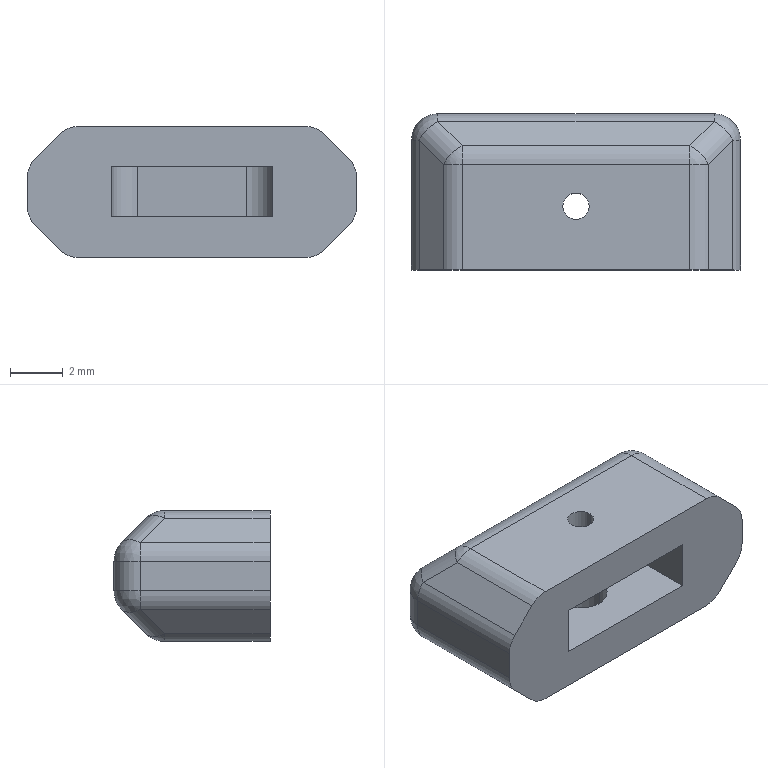Part | NX | features BREP 1 | 1 solid | 49 faces | box 12.444 x 5.907 x 4.95 mm | volume 254.253 mm3 | cylinder 24 | plane 17 | sphere 8 | commonest cylinder face diameters 2 x22 1 x2
STEP:
#1=CARTESIAN_POINT('',(169.303,55.12,-1.9));
#2=VERTEX_POINT('',#1);
#3=CARTESIAN_POINT('',(171.303,55.12,-1.9));
#4=VERTEX_POINT('',#3);
#5=CARTESIAN_POINT('',(170.303,55.12,-1.9));
#6=DIRECTION('',(0.,0.,1.));
#7=DIRECTION('',(1.,0.,0.));
#8=AXIS2_PLACEMENT_3D('',#5,#6,#7);
#9=CIRCLE('',#8,1.);
#10=EDGE_CURVE('',#2,#4,#9,.T.);
#11=ORIENTED_EDGE('',*,*,#10,.T.);
#12=CARTESIAN_POINT('',(171.303,55.12,-3.45));
#13=VERTEX_POINT('',#12);
#14=CARTESIAN_POINT('',(171.303,55.12,1.5));
#15=DIRECTION('',(0.,0.,-1.));
#16=VECTOR('',#15,1000.);
#17=LINE('',#14,#16);
#18=EDGE_CURVE('',#13,#4,#17,.F.);
#19=ORIENTED_EDGE('',*,*,#18,.F.);
#20=CARTESIAN_POINT('',(169.303,55.12,-3.45));
#21=VERTEX_POINT('',#20);
#22=CARTESIAN_POINT('',(170.303,55.12,-3.45));
#23=DIRECTION('',(0.,0.,-1.));
#24=DIRECTION('',(-1.,0.,0.));
#25=AXIS2_PLACEMENT_3D('',#22,#23,#24);
#26=CIRCLE('',#25,1.);
#27=EDGE_CURVE('',#13,#21,#26,.T.);
#28=ORIENTED_EDGE('',*,*,#27,.T.);
#29=CARTESIAN_POINT('',(169.303,55.12,1.5));
#30=DIRECTION('',(0.,0.,-1.));
#31=VECTOR('',#30,1000.);
#32=LINE('',#29,#31);
#33=EDGE_CURVE('',#21,#2,#32,.F.);
#34=ORIENTED_EDGE('',*,*,#33,.T.);
#35=EDGE_LOOP('',(#11,#19,#28,#34));
#36=FACE_BOUND('',#35,.T.);
#37=CARTESIAN_POINT('',(170.303,55.12,1.5));
#38=DIRECTION('',(0.,0.,-1.));
#39=DIRECTION('',(1.,0.,0.));
#40=AXIS2_PLACEMENT_3D('',#37,#38,#39);
#41=CYLINDRICAL_SURFACE('',#40,1.);
#42=ADVANCED_FACE('',(#36),#41,.F.);
#43=CARTESIAN_POINT('',(170.803,55.12,1.5));
#44=VERTEX_POINT('',#43);
#45=CARTESIAN_POINT('',(169.803,55.12,1.5));
#46=VERTEX_POINT('',#45);
#47=CARTESIAN_POINT('',(170.303,55.12,1.5));
#48=DIRECTION('',(0.,0.,-1.));
#49=DIRECTION('',(1.,0.,0.));
#50=AXIS2_PLACEMENT_3D('',#47,#48,#49);
#51=CIRCLE('',#50,0.5);
#52=EDGE_CURVE('',#44,#46,#51,.T.);
#53=ORIENTED_EDGE('',*,*,#52,.F.);
#54=CARTESIAN_POINT('',(170.803,55.12,0.));
#55=VERTEX_POINT('',#54);
#56=CARTESIAN_POINT('',(170.803,55.12,1.5));
#57=DIRECTION('',(0.,0.,-1.));
#58=VECTOR('',#57,1000.);
#59=LINE('',#56,#58);
#60=EDGE_CURVE('',#55,#44,#59,.F.);
#61=ORIENTED_EDGE('',*,*,#60,.F.);
#62=CARTESIAN_POINT('',(169.803,55.12,0.));
#63=VERTEX_POINT('',#62);
#64=CARTESIAN_POINT('',(170.303,55.12,0.));
#65=DIRECTION('',(0.,0.,1.));
#66=DIRECTION('',(1.,0.,0.));
#67=AXIS2_PLACEMENT_3D('',#64,#65,#66);
#68=CIRCLE('',#67,0.5);
#69=EDGE_CURVE('',#63,#55,#68,.T.);
#70=ORIENTED_EDGE('',*,*,#69,.F.);
#71=CARTESIAN_POINT('',(169.803,55.12,1.5));
#72=DIRECTION('',(0.,0.,-1.));
#73=VECTOR('',#72,1000.);
#74=LINE('',#71,#73);
#75=EDGE_CURVE('',#63,#46,#74,.F.);
#76=ORIENTED_EDGE('',*,*,#75,.T.);
#77=EDGE_LOOP('',(#53,#61,#70,#76));
#78=FACE_BOUND('',#77,.T.);
#79=CARTESIAN_POINT('',(170.303,55.12,1.5));
#80=DIRECTION('',(0.,0.,-1.));
#81=DIRECTION('',(1.,0.,0.));
#82=AXIS2_PLACEMENT_3D('',#79,#80,#81);
#83=CYLINDRICAL_SURFACE('',#82,0.5);
#84=ADVANCED_FACE('',(#78),#83,.F.);
#85=CARTESIAN_POINT('',(165.995,52.713,1.5));
#86=VERTEX_POINT('',#85);
#87=CARTESIAN_POINT('',(174.611,52.713,1.5));
#88=VERTEX_POINT('',#87);
#89=CARTESIAN_POINT('',(0.,52.713,1.5));
#90=DIRECTION('',(1.,0.,0.));
#91=VECTOR('',#90,1000.);
#92=LINE('',#89,#91);
#93=EDGE_CURVE('',#86,#88,#92,.T.);
#94=ORIENTED_EDGE('',*,*,#93,.F.);
#95=CARTESIAN_POINT('',(165.288,52.713,1.207));
#96=VERTEX_POINT('',#95);
#97=CARTESIAN_POINT('',(165.995,52.713,0.5));
#98=DIRECTION('',(0.,-1.,0.));
#99=DIRECTION('',(0.,0.,-1.));
#100=AXIS2_PLACEMENT_3D('',#97,#98,#99);
#101=CIRCLE('',#100,1.);
#102=EDGE_CURVE('',#86,#96,#101,.T.);
#103=ORIENTED_EDGE('',*,*,#102,.T.);
#104=CARTESIAN_POINT('',(164.374,52.713,0.2929));
#105=VERTEX_POINT('',#104);
#106=CARTESIAN_POINT('',(154.219,52.713,-9.862));
#107=DIRECTION('',(-0.7071,0.,-0.7071));
#108=VECTOR('',#107,1000.);
#109=LINE('',#106,#108);
#110=EDGE_CURVE('',#96,#105,#109,.T.);
#111=ORIENTED_EDGE('',*,*,#110,.T.);
#112=CARTESIAN_POINT('',(164.081,52.713,-0.4142));
#113=VERTEX_POINT('',#112);
#114=CARTESIAN_POINT('',(165.081,52.713,-0.4142));
#115=DIRECTION('',(0.,-1.,0.));
#116=DIRECTION('',(0.,0.,-1.));
#117=AXIS2_PLACEMENT_3D('',#114,#115,#116);
#118=CIRCLE('',#117,1.);
#119=EDGE_CURVE('',#105,#113,#118,.T.);
#120=ORIENTED_EDGE('',*,*,#119,.T.);
#121=CARTESIAN_POINT('',(164.081,52.713,-1.536));
#122=VERTEX_POINT('',#121);
#123=CARTESIAN_POINT('',(164.081,52.713,-19.725));
#124=DIRECTION('',(0.,0.,1.));
#125=VECTOR('',#124,1000.);
#126=LINE('',#123,#125);
#127=EDGE_CURVE('',#122,#113,#126,.T.);
#128=ORIENTED_EDGE('',*,*,#127,.F.);
#129=CARTESIAN_POINT('',(164.374,52.713,-2.243));
#130=VERTEX_POINT('',#129);
#131=CARTESIAN_POINT('',(165.081,52.713,-1.536));
#132=DIRECTION('',(0.,-1.,0.));
#133=DIRECTION('',(0.,0.,-1.));
#134=AXIS2_PLACEMENT_3D('',#131,#132,#133);
#135=CIRCLE('',#134,1.);
#136=EDGE_CURVE('',#122,#130,#135,.T.);
#137=ORIENTED_EDGE('',*,*,#136,.T.);
#138=CARTESIAN_POINT('',(165.288,52.713,-3.157));
#139=VERTEX_POINT('',#138);
#140=CARTESIAN_POINT('',(172.969,52.713,-10.837));
#141=DIRECTION('',(0.7071,0.,-0.7071));
#142=VECTOR('',#141,1000.);
#143=LINE('',#140,#142);
#144=EDGE_CURVE('',#130,#139,#143,.T.);
#145=ORIENTED_EDGE('',*,*,#144,.T.);
#146=CARTESIAN_POINT('',(165.995,52.713,-3.45));
#147=VERTEX_POINT('',#146);
#148=CARTESIAN_POINT('',(165.995,52.713,-2.45));
#149=DIRECTION('',(0.,-1.,0.));
#150=DIRECTION('',(0.,0.,-1.));
#151=AXIS2_PLACEMENT_3D('',#148,#149,#150);
#152=CIRCLE('',#151,1.);
#153=EDGE_CURVE('',#139,#147,#152,.T.);
#154=ORIENTED_EDGE('',*,*,#153,.T.);
#155=CARTESIAN_POINT('',(174.611,52.713,-3.45));
#156=VERTEX_POINT('',#155);
#157=CARTESIAN_POINT('',(164.081,52.713,-3.45));
#158=DIRECTION('',(-1.,0.,0.));
#159=VECTOR('',#158,1000.);
#160=LINE('',#157,#159);
#161=EDGE_CURVE('',#156,#147,#160,.T.);
#162=ORIENTED_EDGE('',*,*,#161,.F.);
#163=CARTESIAN_POINT('',(175.318,52.713,-3.157));
#164=VERTEX_POINT('',#163);
#165=CARTESIAN_POINT('',(174.611,52.713,-2.45));
#166=DIRECTION('',(0.,-1.,0.));
#167=DIRECTION('',(0.,0.,-1.));
#168=AXIS2_PLACEMENT_3D('',#165,#166,#167);
#169=CIRCLE('',#168,1.);
#170=EDGE_CURVE('',#156,#164,#169,.T.);
#171=ORIENTED_EDGE('',*,*,#170,.T.);
#172=CARTESIAN_POINT('',(176.232,52.713,-2.243));
#173=VERTEX_POINT('',#172);
#174=CARTESIAN_POINT('',(161.416,52.713,-17.059));
#175=DIRECTION('',(0.7071,0.,0.7071));
#176=VECTOR('',#175,1000.);
#177=LINE('',#174,#176);
#178=EDGE_CURVE('',#164,#173,#177,.T.);
#179=ORIENTED_EDGE('',*,*,#178,.T.);
#180=CARTESIAN_POINT('',(176.525,52.713,-1.536));
#181=VERTEX_POINT('',#180);
#182=CARTESIAN_POINT('',(175.525,52.713,-1.536));
#183=DIRECTION('',(0.,-1.,0.));
#184=DIRECTION('',(0.,0.,-1.));
#185=AXIS2_PLACEMENT_3D('',#182,#183,#184);
#186=CIRCLE('',#185,1.);
#187=EDGE_CURVE('',#173,#181,#186,.T.);
#188=ORIENTED_EDGE('',*,*,#187,.T.);
#189=CARTESIAN_POINT('',(176.525,52.713,-0.4142));
#190=VERTEX_POINT('',#189);
#191=CARTESIAN_POINT('',(176.525,52.713,-19.725));
#192=DIRECTION('',(0.,0.,1.));
#193=VECTOR('',#192,1000.);
#194=LINE('',#191,#193);
#195=EDGE_CURVE('',#181,#190,#194,.T.);
#196=ORIENTED_EDGE('',*,*,#195,.T.);
#197=CARTESIAN_POINT('',(176.232,52.713,0.2929));
#198=VERTEX_POINT('',#197);
#199=CARTESIAN_POINT('',(175.525,52.713,-0.4142));
#200=DIRECTION('',(0.,-1.,0.));
#201=DIRECTION('',(0.,0.,-1.));
#202=AXIS2_PLACEMENT_3D('',#199,#200,#201);
#203=CIRCLE('',#202,1.);
#204=EDGE_CURVE('',#190,#198,#203,.T.);
#205=ORIENTED_EDGE('',*,*,#204,.T.);
#206=CARTESIAN_POINT('',(175.318,52.713,1.207));
#207=VERTEX_POINT('',#206);
#208=CARTESIAN_POINT('',(180.166,52.713,-3.64));
#209=DIRECTION('',(-0.7071,0.,0.7071));
#210=VECTOR('',#209,1000.);
#211=LINE('',#208,#210);
#212=EDGE_CURVE('',#198,#207,#211,.T.);
#213=ORIENTED_EDGE('',*,*,#212,.T.);
#214=CARTESIAN_POINT('',(174.611,52.713,0.5));
#215=DIRECTION('',(0.,-1.,0.));
#216=DIRECTION('',(0.,0.,-1.));
#217=AXIS2_PLACEMENT_3D('',#214,#215,#216);
#218=CIRCLE('',#217,1.);
#219=EDGE_CURVE('',#207,#88,#218,.T.);
#220=ORIENTED_EDGE('',*,*,#219,.T.);
#221=EDGE_LOOP('',(#94,#103,#111,#120,#128,#137,#145,#154,#162,#171,#179,#188,#196,#205,#213,#220));
#222=FACE_BOUND('',#221,.T.);
#223=CARTESIAN_POINT('',(173.353,52.713,0.));
#224=VERTEX_POINT('',#223);
#225=CARTESIAN_POINT('',(173.353,52.713,-1.9));
#226=VERTEX_POINT('',#225);
#227=CARTESIAN_POINT('',(173.353,52.713,-19.725));
#228=DIRECTION('',(0.,0.,-1.));
#229=VECTOR('',#228,1000.);
#230=LINE('',#227,#229);
#231=EDGE_CURVE('',#224,#226,#230,.T.);
#232=ORIENTED_EDGE('',*,*,#231,.T.);
#233=CARTESIAN_POINT('',(167.253,52.713,-1.9));
#234=VERTEX_POINT('',#233);
#235=CARTESIAN_POINT('',(164.081,52.713,-1.9));
#236=DIRECTION('',(-1.,0.,0.));
#237=VECTOR('',#236,1000.);
#238=LINE('',#235,#237);
#239=EDGE_CURVE('',#226,#234,#238,.T.);
#240=ORIENTED_EDGE('',*,*,#239,.T.);
#241=CARTESIAN_POINT('',(167.253,52.713,0.));
#242=VERTEX_POINT('',#241);
#243=CARTESIAN_POINT('',(167.253,52.713,-19.725));
#244=DIRECTION('',(0.,0.,1.));
#245=VECTOR('',#244,1000.);
#246=LINE('',#243,#245);
#247=EDGE_CURVE('',#234,#242,#246,.T.);
#248=ORIENTED_EDGE('',*,*,#247,.T.);
#249=CARTESIAN_POINT('',(164.081,52.713,0.));
#250=DIRECTION('',(-1.,0.,0.));
#251=VECTOR('',#250,1000.);
#252=LINE('',#249,#251);
#253=EDGE_CURVE('',#224,#242,#252,.T.);
#254=ORIENTED_EDGE('',*,*,#253,.F.);
#255=EDGE_LOOP('',(#232,#240,#248,#254));
#256=FACE_BOUND('',#255,.T.);
#257=CARTESIAN_POINT('',(164.081,52.713,-19.725));
#258=DIRECTION('',(0.,-1.,0.));
#259=DIRECTION('',(0.,0.,1.));
#260=AXIS2_PLACEMENT_3D('',#257,#258,#259);
#261=PLANE('',#260);
#262=ADVANCED_FACE('',(#222,#256),#261,.T.);
#263=CARTESIAN_POINT('',(176.525,57.62,-1.536));
#264=VERTEX_POINT('',#263);
#265=CARTESIAN_POINT('',(176.525,57.62,-0.4142));
#266=VERTEX_POINT('',#265);
#267=CARTESIAN_POINT('',(176.525,57.62,-19.725));
#268=DIRECTION('',(0.,0.,1.));
#269=VECTOR('',#268,1000.);
#270=LINE('',#267,#269);
#271=EDGE_CURVE('',#264,#266,#270,.T.);
#272=ORIENTED_EDGE('',*,*,#271,.T.);
#273=CARTESIAN_POINT('',(176.525,58.62,-0.4142));
#274=DIRECTION('',(0.,-1.,0.));
#275=VECTOR('',#274,1000.);
#276=LINE('',#273,#275);
#277=EDGE_CURVE('',#266,#190,#276,.T.);
#278=ORIENTED_EDGE('',*,*,#277,.T.);
#279=ORIENTED_EDGE('',*,*,#195,.F.);
#280=CARTESIAN_POINT('',(176.525,58.62,-1.536));
#281=DIRECTION('',(0.,1.,0.));
#282=VECTOR('',#281,1000.);
#283=LINE('',#280,#282);
#284=EDGE_CURVE('',#181,#264,#283,.T.);
#285=ORIENTED_EDGE('',*,*,#284,.T.);
#286=EDGE_LOOP('',(#272,#278,#279,#285));
#287=FACE_BOUND('',#286,.T.);
#288=CARTESIAN_POINT('',(176.525,58.62,-19.725));
#289=DIRECTION('',(1.,0.,0.));
#290=DIRECTION('',(0.,-1.,0.));
#291=AXIS2_PLACEMENT_3D('',#288,#289,#290);
#292=PLANE('',#291);
#293=ADVANCED_FACE('',(#287),#292,.T.);
#294=ORIENTED_EDGE('',*,*,#127,.T.);
#295=CARTESIAN_POINT('',(164.081,57.62,-0.4142));
#296=VERTEX_POINT('',#295);
#297=CARTESIAN_POINT('',(164.081,58.62,-0.4142));
#298=DIRECTION('',(0.,1.,0.));
#299=VECTOR('',#298,1000.);
#300=LINE('',#297,#299);
#301=EDGE_CURVE('',#113,#296,#300,.T.);
#302=ORIENTED_EDGE('',*,*,#301,.T.);
#303=CARTESIAN_POINT('',(164.081,57.62,-1.536));
#304=VERTEX_POINT('',#303);
#305=CARTESIAN_POINT('',(164.081,57.62,-19.725));
#306=DIRECTION('',(0.,0.,-1.));
#307=VECTOR('',#306,1000.);
#308=LINE('',#305,#307);
#309=EDGE_CURVE('',#296,#304,#308,.T.);
#310=ORIENTED_EDGE('',*,*,#309,.T.);
#311=CARTESIAN_POINT('',(164.081,58.62,-1.536));
#312=DIRECTION('',(0.,-1.,0.));
#313=VECTOR('',#312,1000.);
#314=LINE('',#311,#313);
#315=EDGE_CURVE('',#304,#122,#314,.T.);
#316=ORIENTED_EDGE('',*,*,#315,.T.);
#317=EDGE_LOOP('',(#294,#302,#310,#316));
#318=FACE_BOUND('',#317,.T.);
#319=CARTESIAN_POINT('',(164.081,58.62,-19.725));
#320=DIRECTION('',(-1.,0.,0.));
#321=DIRECTION('',(0.,0.,-1.));
#322=AXIS2_PLACEMENT_3D('',#319,#320,#321);
#323=PLANE('',#322);
#324=ADVANCED_FACE('',(#318),#323,.T.);
#325=CARTESIAN_POINT('',(175.525,58.62,-1.536));
#326=VERTEX_POINT('',#325);
#327=CARTESIAN_POINT('',(165.081,58.62,-1.536));
#328=VERTEX_POINT('',#327);
#329=CARTESIAN_POINT('',(164.081,58.62,-1.536));
#330=DIRECTION('',(-1.,0.,0.));
#331=VECTOR('',#330,1000.);
#332=LINE('',#329,#331);
#333=EDGE_CURVE('',#326,#328,#332,.T.);
#334=ORIENTED_EDGE('',*,*,#333,.T.);
#335=CARTESIAN_POINT('',(165.081,58.62,-0.4142));
#336=VERTEX_POINT('',#335);
#337=CARTESIAN_POINT('',(165.081,58.62,-19.725));
#338=DIRECTION('',(0.,0.,1.));
#339=VECTOR('',#338,1000.);
#340=LINE('',#337,#339);
#341=EDGE_CURVE('',#328,#336,#340,.T.);
#342=ORIENTED_EDGE('',*,*,#341,.T.);
#343=CARTESIAN_POINT('',(175.525,58.62,-0.4142));
#344=VERTEX_POINT('',#343);
#345=CARTESIAN_POINT('',(164.081,58.62,-0.4142));
#346=DIRECTION('',(1.,0.,0.));
#347=VECTOR('',#346,1000.);
#348=LINE('',#345,#347);
#349=EDGE_CURVE('',#336,#344,#348,.T.);
#350=ORIENTED_EDGE('',*,*,#349,.T.);
#351=CARTESIAN_POINT('',(175.525,58.62,-19.725));
#352=DIRECTION('',(0.,0.,-1.));
#353=VECTOR('',#352,1000.);
#354=LINE('',#351,#353);
#355=EDGE_CURVE('',#344,#326,#354,.T.);
#356=ORIENTED_EDGE('',*,*,#355,.T.);
#357=EDGE_LOOP('',(#334,#342,#350,#356));
#358=FACE_BOUND('',#357,.T.);
#359=CARTESIAN_POINT('',(164.081,58.62,-19.725));
#360=DIRECTION('',(0.,1.,0.));
#361=DIRECTION('',(-1.,0.,0.));
#362=AXIS2_PLACEMENT_3D('',#359,#360,#361);
#363=PLANE('',#362);
#364=ADVANCED_FACE('',(#358),#363,.T.);
#365=CARTESIAN_POINT('',(165.995,56.705,-3.45));
#366=VERTEX_POINT('',#365);
#367=CARTESIAN_POINT('',(174.611,56.705,-3.45));
#368=VERTEX_POINT('',#367);
#369=CARTESIAN_POINT('',(175.025,56.705,-3.45));
#370=DIRECTION('',(1.,0.,0.));
#371=VECTOR('',#370,1000.);
#372=LINE('',#369,#371);
#373=EDGE_CURVE('',#366,#368,#372,.T.);
#374=ORIENTED_EDGE('',*,*,#373,.T.);
#375=CARTESIAN_POINT('',(174.611,52.713,-3.45));
#376=DIRECTION('',(0.,-1.,0.));
#377=VECTOR('',#376,1000.);
#378=LINE('',#375,#377);
#379=EDGE_CURVE('',#368,#156,#378,.T.);
#380=ORIENTED_EDGE('',*,*,#379,.T.);
#381=ORIENTED_EDGE('',*,*,#161,.T.);
#382=CARTESIAN_POINT('',(165.995,57.12,-3.45));
#383=DIRECTION('',(0.,1.,0.));
#384=VECTOR('',#383,1000.);
#385=LINE('',#382,#384);
#386=EDGE_CURVE('',#147,#366,#385,.T.);
#387=ORIENTED_EDGE('',*,*,#386,.T.);
#388=EDGE_LOOP('',(#374,#380,#381,#387));
#389=FACE_BOUND('',#388,.T.);
#390=CARTESIAN_POINT('',(170.303,55.12,-3.45));
#391=DIRECTION('',(0.,0.,-1.));
#392=DIRECTION('',(-1.,0.,0.));
#393=AXIS2_PLACEMENT_3D('',#390,#391,#392);
#394=CIRCLE('',#393,1.);
#395=EDGE_CURVE('',#21,#13,#394,.T.);
#396=ORIENTED_EDGE('',*,*,#395,.F.);
#397=ORIENTED_EDGE('',*,*,#27,.F.);
#398=EDGE_LOOP('',(#396,#397));
#399=FACE_BOUND('',#398,.T.);
#400=CARTESIAN_POINT('',(367.911,31.929,-3.45));
#401=DIRECTION('',(0.,0.,1.));
#402=DIRECTION('',(-1.,0.,0.));
#403=AXIS2_PLACEMENT_3D('',#400,#401,#402);
#404=PLANE('',#403);
#405=ADVANCED_FACE('',(#389,#399),#404,.F.);
#406=CARTESIAN_POINT('',(174.611,56.705,1.5));
#407=VERTEX_POINT('',#406);
#408=CARTESIAN_POINT('',(165.995,56.705,1.5));
#409=VERTEX_POINT('',#408);
#410=CARTESIAN_POINT('',(0.,56.705,1.5));
#411=DIRECTION('',(-1.,0.,0.));
#412=VECTOR('',#411,1000.);
#413=LINE('',#410,#412);
#414=EDGE_CURVE('',#407,#409,#413,.T.);
#415=ORIENTED_EDGE('',*,*,#414,.T.);
#416=CARTESIAN_POINT('',(165.995,0.,1.5));
#417=DIRECTION('',(0.,-1.,0.));
#418=VECTOR('',#417,1000.);
#419=LINE('',#416,#418);
#420=EDGE_CURVE('',#409,#86,#419,.T.);
#421=ORIENTED_EDGE('',*,*,#420,.T.);
#422=ORIENTED_EDGE('',*,*,#93,.T.);
#423=CARTESIAN_POINT('',(174.611,0.,1.5));
#424=DIRECTION('',(0.,1.,0.));
#425=VECTOR('',#424,1000.);
#426=LINE('',#423,#425);
#427=EDGE_CURVE('',#88,#407,#426,.T.);
#428=ORIENTED_EDGE('',*,*,#427,.T.);
#429=EDGE_LOOP('',(#415,#421,#422,#428));
#430=FACE_BOUND('',#429,.T.);
#431=CARTESIAN_POINT('',(170.303,55.12,1.5));
#432=DIRECTION('',(0.,0.,-1.));
#433=DIRECTION('',(1.,0.,0.));
#434=AXIS2_PLACEMENT_3D('',#431,#432,#433);
#435=CIRCLE('',#434,0.5);
#436=EDGE_CURVE('',#46,#44,#435,.T.);
#437=ORIENTED_EDGE('',*,*,#436,.T.);
#438=ORIENTED_EDGE('',*,*,#52,.T.);
#439=EDGE_LOOP('',(#437,#438));
#440=FACE_BOUND('',#439,.T.);
#441=CARTESIAN_POINT('',(0.,0.,1.5));
#442=DIRECTION('',(0.,0.,1.));
#443=DIRECTION('',(-1.,0.,0.));
#444=AXIS2_PLACEMENT_3D('',#441,#442,#443);
#445=PLANE('',#444);
#446=ADVANCED_FACE('',(#430,#440),#445,.T.);
#447=CARTESIAN_POINT('',(176.232,57.62,0.2929));
#448=VERTEX_POINT('',#447);
#449=CARTESIAN_POINT('',(175.318,56.705,1.207));
#450=VERTEX_POINT('',#449);
#451=CARTESIAN_POINT('',(156.221,37.608,20.304));
#452=DIRECTION('',(-0.5774,-0.5774,0.5774));
#453=VECTOR('',#452,1000.);
#454=LINE('',#451,#453);
#455=EDGE_CURVE('',#448,#450,#454,.T.);
#456=ORIENTED_EDGE('',*,*,#455,.T.);
#457=CARTESIAN_POINT('',(175.318,0.,1.207));
#458=DIRECTION('',(0.,-1.,0.));
#459=VECTOR('',#458,1000.);
#460=LINE('',#457,#459);
#461=EDGE_CURVE('',#450,#207,#460,.T.);
#462=ORIENTED_EDGE('',*,*,#461,.T.);
#463=ORIENTED_EDGE('',*,*,#212,.F.);
#464=CARTESIAN_POINT('',(176.232,0.,0.2929));
#465=DIRECTION('',(0.,1.,0.));
#466=VECTOR('',#465,1000.);
#467=LINE('',#464,#466);
#468=EDGE_CURVE('',#198,#448,#467,.T.);
#469=ORIENTED_EDGE('',*,*,#468,.T.);
#470=EDGE_LOOP('',(#456,#462,#463,#469));
#471=FACE_BOUND('',#470,.T.);
#472=CARTESIAN_POINT('',(175.025,0.,1.5));
#473=DIRECTION('',(-0.7071,0.,-0.7071));
#474=DIRECTION('',(0.7071,0.,-0.7071));
#475=AXIS2_PLACEMENT_3D('',#472,#473,#474);
#476=PLANE('',#475);
#477=ADVANCED_FACE('',(#471),#476,.F.);
#478=ORIENTED_EDGE('',*,*,#178,.F.);
#479=CARTESIAN_POINT('',(175.318,56.705,-3.157));
#480=VERTEX_POINT('',#479);
#481=CARTESIAN_POINT('',(175.318,57.12,-3.157));
#482=DIRECTION('',(0.,1.,0.));
#483=VECTOR('',#482,1000.);
#484=LINE('',#481,#483);
#485=EDGE_CURVE('',#164,#480,#484,.T.);
#486=ORIENTED_EDGE('',*,*,#485,.T.);
#487=CARTESIAN_POINT('',(176.232,57.62,-2.243));
#488=VERTEX_POINT('',#487);
#489=CARTESIAN_POINT('',(166.864,48.251,-11.611));
#490=DIRECTION('',(0.5774,0.5774,0.5774));
#491=VECTOR('',#490,1000.);
#492=LINE('',#489,#491);
#493=EDGE_CURVE('',#480,#488,#492,.T.);
#494=ORIENTED_EDGE('',*,*,#493,.T.);
#495=CARTESIAN_POINT('',(176.232,31.929,-2.243));
#496=DIRECTION('',(0.,-1.,0.));
#497=VECTOR('',#496,1000.);
#498=LINE('',#495,#497);
#499=EDGE_CURVE('',#488,#173,#498,.T.);
#500=ORIENTED_EDGE('',*,*,#499,.T.);
#501=EDGE_LOOP('',(#478,#486,#494,#500));
#502=FACE_BOUND('',#501,.T.);
#503=CARTESIAN_POINT('',(175.025,31.929,-3.45));
#504=DIRECTION('',(0.7071,0.,-0.7071));
#505=DIRECTION('',(0.,1.,0.));
#506=AXIS2_PLACEMENT_3D('',#503,#504,#505);
#507=PLANE('',#506);
#508=ADVANCED_FACE('',(#502),#507,.T.);
#509=ORIENTED_EDGE('',*,*,#110,.F.);
#510=CARTESIAN_POINT('',(165.288,56.705,1.207));
#511=VERTEX_POINT('',#510);
#512=CARTESIAN_POINT('',(165.288,0.,1.207));
#513=DIRECTION('',(0.,1.,0.));
#514=VECTOR('',#513,1000.);
#515=LINE('',#512,#514);
#516=EDGE_CURVE('',#96,#511,#515,.T.);
#517=ORIENTED_EDGE('',*,*,#516,.T.);
#518=CARTESIAN_POINT('',(164.374,57.62,0.2929));
#519=VERTEX_POINT('',#518);
#520=CARTESIAN_POINT('',(184.385,37.608,20.304));
#521=DIRECTION('',(-0.5774,0.5774,-0.5774));
#522=VECTOR('',#521,1000.);
#523=LINE('',#520,#522);
#524=EDGE_CURVE('',#511,#519,#523,.T.);
#525=ORIENTED_EDGE('',*,*,#524,.T.);
#526=CARTESIAN_POINT('',(164.374,0.,0.2929));
#527=DIRECTION('',(0.,-1.,0.));
#528=VECTOR('',#527,1000.);
#529=LINE('',#526,#528);
#530=EDGE_CURVE('',#519,#105,#529,.T.);
#531=ORIENTED_EDGE('',*,*,#530,.T.);
#532=EDGE_LOOP('',(#509,#517,#525,#531));
#533=FACE_BOUND('',#532,.T.);
#534=CARTESIAN_POINT('',(165.581,0.,1.5));
#535=DIRECTION('',(0.7071,0.,-0.7071));
#536=DIRECTION('',(0.,1.,0.));
#537=AXIS2_PLACEMENT_3D('',#534,#535,#536);
#538=PLANE('',#537);
#539=ADVANCED_FACE('',(#533),#538,.F.);
#540=CARTESIAN_POINT('',(164.374,57.62,-2.243));
#541=VERTEX_POINT('',#540);
#542=CARTESIAN_POINT('',(165.288,56.705,-3.157));
#543=VERTEX_POINT('',#542);
#544=CARTESIAN_POINT('',(173.742,48.251,-11.611));
#545=DIRECTION('',(0.5774,-0.5774,-0.5774));
#546=VECTOR('',#545,1000.);
#547=LINE('',#544,#546);
#548=EDGE_CURVE('',#541,#543,#547,.T.);
#549=ORIENTED_EDGE('',*,*,#548,.T.);
#550=CARTESIAN_POINT('',(165.288,52.713,-3.157));
#551=DIRECTION('',(0.,-1.,0.));
#552=VECTOR('',#551,1000.);
#553=LINE('',#550,#552);
#554=EDGE_CURVE('',#543,#139,#553,.T.);
#555=ORIENTED_EDGE('',*,*,#554,.T.);
#556=ORIENTED_EDGE('',*,*,#144,.F.);
#557=CARTESIAN_POINT('',(164.374,31.929,-2.243));
#558=DIRECTION('',(0.,1.,0.));
#559=VECTOR('',#558,1000.);
#560=LINE('',#557,#559);
#561=EDGE_CURVE('',#130,#541,#560,.T.);
#562=ORIENTED_EDGE('',*,*,#561,.T.);
#563=EDGE_LOOP('',(#549,#555,#556,#562));
#564=FACE_BOUND('',#563,.T.);
#565=CARTESIAN_POINT('',(165.581,31.929,-3.45));
#566=DIRECTION('',(-0.7071,0.,-0.7071));
#567=DIRECTION('',(0.7071,0.,-0.7071));
#568=AXIS2_PLACEMENT_3D('',#565,#566,#567);
#569=PLANE('',#568);
#570=ADVANCED_FACE('',(#564),#569,.T.);
#571=CARTESIAN_POINT('',(165.081,58.327,0.2929));
#572=VERTEX_POINT('',#571);
#573=CARTESIAN_POINT('',(165.995,57.412,1.207));
#574=VERTEX_POINT('',#573);
#575=CARTESIAN_POINT('',(110.859,112.549,-53.929));
#576=DIRECTION('',(0.5774,-0.5774,0.5774));
#577=VECTOR('',#576,1000.);
#578=LINE('',#575,#577);
#579=EDGE_CURVE('',#572,#574,#578,.T.);
#580=ORIENTED_EDGE('',*,*,#579,.T.);
#581=CARTESIAN_POINT('',(174.611,57.412,1.207));
#582=VERTEX_POINT('',#581);
#583=CARTESIAN_POINT('',(0.,57.412,1.207));
#584=DIRECTION('',(1.,0.,0.));
#585=VECTOR('',#584,1000.);
#586=LINE('',#583,#585);
#587=EDGE_CURVE('',#574,#582,#586,.T.);
#588=ORIENTED_EDGE('',*,*,#587,.T.);
#589=CARTESIAN_POINT('',(175.525,58.327,0.2929));
#590=VERTEX_POINT('',#589);
#591=CARTESIAN_POINT('',(116.212,-0.9865,59.606));
#592=DIRECTION('',(0.5774,0.5774,-0.5774));
#593=VECTOR('',#592,1000.);
#594=LINE('',#591,#593);
#595=EDGE_CURVE('',#582,#590,#594,.T.);
#596=ORIENTED_EDGE('',*,*,#595,.T.);
#597=CARTESIAN_POINT('',(0.,58.327,0.2929));
#598=DIRECTION('',(-1.,0.,0.));
#599=VECTOR('',#598,1000.);
#600=LINE('',#597,#599);
#601=EDGE_CURVE('',#590,#572,#600,.T.);
#602=ORIENTED_EDGE('',*,*,#601,.T.);
#603=EDGE_LOOP('',(#580,#588,#596,#602));
#604=FACE_BOUND('',#603,.T.);
#605=CARTESIAN_POINT('',(0.,57.12,1.5));
#606=DIRECTION('',(0.,-0.7071,-0.7071));
#607=DIRECTION('',(0.,-0.7071,0.7071));
#608=AXIS2_PLACEMENT_3D('',#605,#606,#607);
#609=PLANE('',#608);
#610=ADVANCED_FACE('',(#604),#609,.F.);
#611=CARTESIAN_POINT('',(175.525,58.327,-2.243));
#612=VERTEX_POINT('',#611);
#613=CARTESIAN_POINT('',(174.611,57.412,-3.157));
#614=VERTEX_POINT('',#613);
#615=CARTESIAN_POINT('',(238.849,121.65,61.081));
#616=DIRECTION('',(-0.5774,-0.5774,-0.5774));
#617=VECTOR('',#616,1000.);
#618=LINE('',#615,#617);
#619=EDGE_CURVE('',#612,#614,#618,.T.);
#620=ORIENTED_EDGE('',*,*,#619,.T.);
#621=CARTESIAN_POINT('',(165.995,57.412,-3.157));
#622=VERTEX_POINT('',#621);
#623=CARTESIAN_POINT('',(165.581,57.412,-3.157));
#624=DIRECTION('',(-1.,0.,0.));
#625=VECTOR('',#624,1000.);
#626=LINE('',#623,#625);
#627=EDGE_CURVE('',#614,#622,#626,.T.);
#628=ORIENTED_EDGE('',*,*,#627,.T.);
#629=CARTESIAN_POINT('',(165.081,58.327,-2.243));
#630=VERTEX_POINT('',#629);
#631=CARTESIAN_POINT('',(233.496,-10.088,-70.657));
#632=DIRECTION('',(-0.5774,0.5774,0.5774));
#633=VECTOR('',#632,1000.);
#634=LINE('',#631,#633);
#635=EDGE_CURVE('',#622,#630,#634,.T.);
#636=ORIENTED_EDGE('',*,*,#635,.T.);
#637=CARTESIAN_POINT('',(367.911,58.327,-2.243));
#638=DIRECTION('',(1.,0.,0.));
#639=VECTOR('',#638,1000.);
#640=LINE('',#637,#639);
#641=EDGE_CURVE('',#630,#612,#640,.T.);
#642=ORIENTED_EDGE('',*,*,#641,.T.);
#643=EDGE_LOOP('',(#620,#628,#636,#642));
#644=FACE_BOUND('',#643,.T.);
#645=CARTESIAN_POINT('',(367.911,57.12,-3.45));
#646=DIRECTION('',(0.,0.7071,-0.7071));
#647=DIRECTION('',(1.,0.,0.));
#648=AXIS2_PLACEMENT_3D('',#645,#646,#647);
#649=PLANE('',#648);
#650=ADVANCED_FACE('',(#644),#649,.T.);
#651=CARTESIAN_POINT('',(174.611,56.705,-2.45));
#652=DIRECTION('',(0.,1.,0.));
#653=DIRECTION('',(-1.,0.,0.));
#654=AXIS2_PLACEMENT_3D('',#651,#652,#653);
#655=CIRCLE('',#654,1.);
#656=EDGE_CURVE('',#480,#368,#655,.T.);
#657=ORIENTED_EDGE('',*,*,#656,.F.);
#658=ORIENTED_EDGE('',*,*,#485,.F.);
#659=ORIENTED_EDGE('',*,*,#170,.F.);
#660=ORIENTED_EDGE('',*,*,#379,.F.);
#661=EDGE_LOOP('',(#657,#658,#659,#660));
#662=FACE_BOUND('',#661,.T.);
#663=CARTESIAN_POINT('',(174.611,31.929,-2.45));
#664=DIRECTION('',(0.,1.,0.));
#665=DIRECTION('',(0.,0.,-1.));
#666=AXIS2_PLACEMENT_3D('',#663,#664,#665);
#667=CYLINDRICAL_SURFACE('',#666,1.);
#668=ADVANCED_FACE('',(#662),#667,.T.);
#669=CARTESIAN_POINT('',(174.611,56.705,-2.45));
#670=DIRECTION('',(0.5774,0.5774,0.5774));
#671=DIRECTION('',(-0.7071,0.,0.7071));
#672=AXIS2_PLACEMENT_3D('',#669,#670,#671);
#673=CIRCLE('',#672,1.);
#674=EDGE_CURVE('',#480,#614,#673,.T.);
#675=ORIENTED_EDGE('',*,*,#674,.F.);
#676=ORIENTED_EDGE('',*,*,#656,.T.);
#677=CARTESIAN_POINT('',(174.611,56.705,-2.45));
#678=DIRECTION('',(-1.,0.,0.));
#679=DIRECTION('',(0.,1.,0.));
#680=AXIS2_PLACEMENT_3D('',#677,#678,#679);
#681=CIRCLE('',#680,1.);
#682=EDGE_CURVE('',#614,#368,#681,.T.);
#683=ORIENTED_EDGE('',*,*,#682,.F.);
#684=EDGE_LOOP('',(#675,#676,#683));
#685=FACE_BOUND('',#684,.T.);
#686=CARTESIAN_POINT('',(174.611,56.705,-2.45));
#687=DIRECTION('',(0.,0.,-1.));
#688=DIRECTION('',(-1.,0.,0.));
#689=AXIS2_PLACEMENT_3D('',#686,#687,#688);
#690=SPHERICAL_SURFACE('',#689,1.);
#691=ADVANCED_FACE('',(#685),#690,.T.);
#692=ORIENTED_EDGE('',*,*,#153,.F.);
#693=ORIENTED_EDGE('',*,*,#554,.F.);
#694=CARTESIAN_POINT('',(165.995,56.705,-2.45));
#695=DIRECTION('',(0.,1.,0.));
#696=DIRECTION('',(-1.,0.,0.));
#697=AXIS2_PLACEMENT_3D('',#694,#695,#696);
#698=CIRCLE('',#697,1.);
#699=EDGE_CURVE('',#366,#543,#698,.T.);
#700=ORIENTED_EDGE('',*,*,#699,.F.);
#701=ORIENTED_EDGE('',*,*,#386,.F.);
#702=EDGE_LOOP('',(#692,#693,#700,#701));
#703=FACE_BOUND('',#702,.T.);
#704=CARTESIAN_POINT('',(165.995,31.929,-2.45));
#705=DIRECTION('',(0.,-1.,0.));
#706=DIRECTION('',(0.,0.,1.));
#707=AXIS2_PLACEMENT_3D('',#704,#705,#706);
#708=CYLINDRICAL_SURFACE('',#707,1.);
#709=ADVANCED_FACE('',(#703),#708,.T.);
#710=ORIENTED_EDGE('',*,*,#682,.T.);
#711=ORIENTED_EDGE('',*,*,#373,.F.);
#712=CARTESIAN_POINT('',(165.995,56.705,-2.45));
#713=DIRECTION('',(-1.,0.,0.));
#714=DIRECTION('',(0.,0.,1.));
#715=AXIS2_PLACEMENT_3D('',#712,#713,#714);
#716=CIRCLE('',#715,1.);
#717=EDGE_CURVE('',#622,#366,#716,.T.);
#718=ORIENTED_EDGE('',*,*,#717,.F.);
#719=ORIENTED_EDGE('',*,*,#627,.F.);
#720=EDGE_LOOP('',(#710,#711,#718,#719));
#721=FACE_BOUND('',#720,.T.);
#722=CARTESIAN_POINT('',(367.911,56.705,-2.45));
#723=DIRECTION('',(-1.,0.,0.));
#724=DIRECTION('',(0.,0.,-1.));
#725=AXIS2_PLACEMENT_3D('',#722,#723,#724);
#726=CYLINDRICAL_SURFACE('',#725,1.);
#727=ADVANCED_FACE('',(#721),#726,.T.);
#728=ORIENTED_EDGE('',*,*,#674,.T.);
#729=ORIENTED_EDGE('',*,*,#619,.F.);
#730=CARTESIAN_POINT('',(175.525,57.62,-1.536));
#731=DIRECTION('',(0.5774,0.5774,0.5774));
#732=DIRECTION('',(0.7071,0.,-0.7071));
#733=AXIS2_PLACEMENT_3D('',#730,#731,#732);
#734=CIRCLE('',#733,1.);
#735=EDGE_CURVE('',#488,#612,#734,.T.);
#736=ORIENTED_EDGE('',*,*,#735,.F.);
#737=ORIENTED_EDGE('',*,*,#493,.F.);
#738=EDGE_LOOP('',(#728,#729,#736,#737));
#739=FACE_BOUND('',#738,.T.);
#740=CARTESIAN_POINT('',(166.157,48.251,-10.904));
#741=DIRECTION('',(0.5774,0.5774,0.5774));
#742=DIRECTION('',(-0.7071,0.,0.7071));
#743=AXIS2_PLACEMENT_3D('',#740,#741,#742);
#744=CYLINDRICAL_SURFACE('',#743,1.);
#745=ADVANCED_FACE('',(#739),#744,.T.);
#746=ORIENTED_EDGE('',*,*,#187,.F.);
#747=ORIENTED_EDGE('',*,*,#499,.F.);
#748=CARTESIAN_POINT('',(175.525,57.62,-1.536));
#749=DIRECTION('',(0.,1.,0.));
#750=DIRECTION('',(0.,0.,1.));
#751=AXIS2_PLACEMENT_3D('',#748,#749,#750);
#752=CIRCLE('',#751,1.);
#753=EDGE_CURVE('',#264,#488,#752,.T.);
#754=ORIENTED_EDGE('',*,*,#753,.F.);
#755=ORIENTED_EDGE('',*,*,#284,.F.);
#756=EDGE_LOOP('',(#746,#747,#754,#755));
#757=FACE_BOUND('',#756,.T.);
#758=CARTESIAN_POINT('',(175.525,58.62,-1.536));
#759=DIRECTION('',(0.,1.,0.));
#760=DIRECTION('',(0.,0.,-1.));
#761=AXIS2_PLACEMENT_3D('',#758,#759,#760);
#762=CYLINDRICAL_SURFACE('',#761,1.);
#763=ADVANCED_FACE('',(#757),#762,.T.);
#764=ORIENTED_EDGE('',*,*,#717,.T.);
#765=ORIENTED_EDGE('',*,*,#699,.T.);
#766=CARTESIAN_POINT('',(165.995,56.705,-2.45));
#767=DIRECTION('',(-0.5774,0.5774,0.5774));
#768=DIRECTION('',(-0.7071,0.,-0.7071));
#769=AXIS2_PLACEMENT_3D('',#766,#767,#768);
#770=CIRCLE('',#769,1.);
#771=EDGE_CURVE('',#622,#543,#770,.T.);
#772=ORIENTED_EDGE('',*,*,#771,.F.);
#773=EDGE_LOOP('',(#764,#765,#772));
#774=FACE_BOUND('',#773,.T.);
#775=CARTESIAN_POINT('',(165.995,56.705,-2.45));
#776=DIRECTION('',(0.,0.,-1.));
#777=DIRECTION('',(-1.,0.,0.));
#778=AXIS2_PLACEMENT_3D('',#775,#776,#777);
#779=SPHERICAL_SURFACE('',#778,1.);
#780=ADVANCED_FACE('',(#774),#779,.T.);
#781=ORIENTED_EDGE('',*,*,#753,.T.);
#782=ORIENTED_EDGE('',*,*,#735,.T.);
#783=CARTESIAN_POINT('',(175.525,57.62,-1.536));
#784=DIRECTION('',(-1.,0.,0.));
#785=DIRECTION('',(0.,0.,-1.));
#786=AXIS2_PLACEMENT_3D('',#783,#784,#785);
#787=CIRCLE('',#786,1.);
#788=EDGE_CURVE('',#326,#612,#787,.T.);
#789=ORIENTED_EDGE('',*,*,#788,.F.);
#790=CARTESIAN_POINT('',(175.525,57.62,-1.536));
#791=DIRECTION('',(0.,0.,1.));
#792=DIRECTION('',(-1.,0.,0.));
#793=AXIS2_PLACEMENT_3D('',#790,#791,#792);
#794=CIRCLE('',#793,1.);
#795=EDGE_CURVE('',#264,#326,#794,.T.);
#796=ORIENTED_EDGE('',*,*,#795,.F.);
#797=EDGE_LOOP('',(#781,#782,#789,#796));
#798=FACE_BOUND('',#797,.T.);
#799=CARTESIAN_POINT('',(175.525,57.62,-1.536));
#800=DIRECTION('',(0.,0.,-1.));
#801=DIRECTION('',(-1.,0.,0.));
#802=AXIS2_PLACEMENT_3D('',#799,#800,#801);
#803=SPHERICAL_SURFACE('',#802,1.);
#804=ADVANCED_FACE('',(#798),#803,.T.);
#805=ORIENTED_EDGE('',*,*,#136,.F.);
#806=ORIENTED_EDGE('',*,*,#315,.F.);
#807=CARTESIAN_POINT('',(165.081,57.62,-1.536));
#808=DIRECTION('',(0.,1.,0.));
#809=DIRECTION('',(-1.,0.,0.));
#810=AXIS2_PLACEMENT_3D('',#807,#808,#809);
#811=CIRCLE('',#810,1.);
#812=EDGE_CURVE('',#541,#304,#811,.T.);
#813=ORIENTED_EDGE('',*,*,#812,.F.);
#814=ORIENTED_EDGE('',*,*,#561,.F.);
#815=EDGE_LOOP('',(#805,#806,#813,#814));
#816=FACE_BOUND('',#815,.T.);
#817=CARTESIAN_POINT('',(165.081,58.62,-1.536));
#818=DIRECTION('',(0.,-1.,0.));
#819=DIRECTION('',(0.,0.,1.));
#820=AXIS2_PLACEMENT_3D('',#817,#818,#819);
#821=CYLINDRICAL_SURFACE('',#820,1.);
#822=ADVANCED_FACE('',(#816),#821,.T.);
#823=ORIENTED_EDGE('',*,*,#771,.T.);
#824=ORIENTED_EDGE('',*,*,#548,.F.);
#825=CARTESIAN_POINT('',(165.081,57.62,-1.536));
#826=DIRECTION('',(-0.5774,0.5774,0.5774));
#827=DIRECTION('',(0.7071,0.,0.7071));
#828=AXIS2_PLACEMENT_3D('',#825,#826,#827);
#829=CIRCLE('',#828,1.);
#830=EDGE_CURVE('',#630,#541,#829,.T.);
#831=ORIENTED_EDGE('',*,*,#830,.F.);
#832=ORIENTED_EDGE('',*,*,#635,.F.);
#833=EDGE_LOOP('',(#823,#824,#831,#832));
#834=FACE_BOUND('',#833,.T.);
#835=CARTESIAN_POINT('',(174.449,48.251,-10.904));
#836=DIRECTION('',(0.5774,-0.5774,-0.5774));
#837=DIRECTION('',(0.7071,0.,0.7071));
#838=AXIS2_PLACEMENT_3D('',#835,#836,#837);
#839=CYLINDRICAL_SURFACE('',#838,1.);
#840=ADVANCED_FACE('',(#834),#839,.T.);
#841=ORIENTED_EDGE('',*,*,#788,.T.);
#842=ORIENTED_EDGE('',*,*,#641,.F.);
#843=CARTESIAN_POINT('',(165.081,57.62,-1.536));
#844=DIRECTION('',(-1.,0.,0.));
#845=DIRECTION('',(0.,0.,1.));
#846=AXIS2_PLACEMENT_3D('',#843,#844,#845);
#847=CIRCLE('',#846,1.);
#848=EDGE_CURVE('',#328,#630,#847,.T.);
#849=ORIENTED_EDGE('',*,*,#848,.F.);
#850=ORIENTED_EDGE('',*,*,#333,.F.);
#851=EDGE_LOOP('',(#841,#842,#849,#850));
#852=FACE_BOUND('',#851,.T.);
#853=CARTESIAN_POINT('',(164.081,57.62,-1.536));
#854=DIRECTION('',(-1.,0.,0.));
#855=DIRECTION('',(0.,0.,-1.));
#856=AXIS2_PLACEMENT_3D('',#853,#854,#855);
#857=CYLINDRICAL_SURFACE('',#856,1.);
#858=ADVANCED_FACE('',(#852),#857,.T.);
#859=ORIENTED_EDGE('',*,*,#795,.T.);
#860=ORIENTED_EDGE('',*,*,#355,.F.);
#861=CARTESIAN_POINT('',(175.525,57.62,-0.4142));
#862=DIRECTION('',(0.,0.,1.));
#863=DIRECTION('',(0.,-1.,0.));
#864=AXIS2_PLACEMENT_3D('',#861,#862,#863);
#865=CIRCLE('',#864,1.);
#866=EDGE_CURVE('',#266,#344,#865,.T.);
#867=ORIENTED_EDGE('',*,*,#866,.F.);
#868=ORIENTED_EDGE('',*,*,#271,.F.);
#869=EDGE_LOOP('',(#859,#860,#867,#868));
#870=FACE_BOUND('',#869,.T.);
#871=CARTESIAN_POINT('',(175.525,57.62,-19.725));
#872=DIRECTION('',(0.,0.,1.));
#873=DIRECTION('',(-1.,0.,0.));
#874=AXIS2_PLACEMENT_3D('',#871,#872,#873);
#875=CYLINDRICAL_SURFACE('',#874,1.);
#876=ADVANCED_FACE('',(#870),#875,.T.);
#877=ORIENTED_EDGE('',*,*,#204,.F.);
#878=ORIENTED_EDGE('',*,*,#277,.F.);
#879=CARTESIAN_POINT('',(175.525,57.62,-0.4142));
#880=DIRECTION('',(0.,1.,0.));
#881=DIRECTION('',(-1.,0.,0.));
#882=AXIS2_PLACEMENT_3D('',#879,#880,#881);
#883=CIRCLE('',#882,1.);
#884=EDGE_CURVE('',#448,#266,#883,.T.);
#885=ORIENTED_EDGE('',*,*,#884,.F.);
#886=ORIENTED_EDGE('',*,*,#468,.F.);
#887=EDGE_LOOP('',(#877,#878,#885,#886));
#888=FACE_BOUND('',#887,.T.);
#889=CARTESIAN_POINT('',(175.525,58.62,-0.4142));
#890=DIRECTION('',(0.,1.,0.));
#891=DIRECTION('',(0.,0.,-1.));
#892=AXIS2_PLACEMENT_3D('',#889,#890,#891);
#893=CYLINDRICAL_SURFACE('',#892,1.);
#894=ADVANCED_FACE('',(#888),#893,.T.);
#895=ORIENTED_EDGE('',*,*,#830,.T.);
#896=ORIENTED_EDGE('',*,*,#812,.T.);
#897=CARTESIAN_POINT('',(165.081,57.62,-1.536));
#898=DIRECTION('',(0.,0.,1.));
#899=DIRECTION('',(0.,1.,0.));
#900=AXIS2_PLACEMENT_3D('',#897,#898,#899);
#901=CIRCLE('',#900,1.);
#902=EDGE_CURVE('',#328,#304,#901,.T.);
#903=ORIENTED_EDGE('',*,*,#902,.F.);
#904=ORIENTED_EDGE('',*,*,#848,.T.);
#905=EDGE_LOOP('',(#895,#896,#903,#904));
#906=FACE_BOUND('',#905,.T.);
#907=CARTESIAN_POINT('',(165.081,57.62,-1.536));
#908=DIRECTION('',(0.,0.,-1.));
#909=DIRECTION('',(-1.,0.,0.));
#910=AXIS2_PLACEMENT_3D('',#907,#908,#909);
#911=SPHERICAL_SURFACE('',#910,1.);
#912=ADVANCED_FACE('',(#906),#911,.T.);
#913=ORIENTED_EDGE('',*,*,#884,.T.);
#914=ORIENTED_EDGE('',*,*,#866,.T.);
#915=CARTESIAN_POINT('',(175.525,57.62,-0.4142));
#916=DIRECTION('',(-1.,0.,0.));
#917=DIRECTION('',(0.,0.,-1.));
#918=AXIS2_PLACEMENT_3D('',#915,#916,#917);
#919=CIRCLE('',#918,1.);
#920=EDGE_CURVE('',#590,#344,#919,.T.);
#921=ORIENTED_EDGE('',*,*,#920,.F.);
#922=CARTESIAN_POINT('',(175.525,57.62,-0.4142));
#923=DIRECTION('',(-0.5774,-0.5774,0.5774));
#924=DIRECTION('',(-0.7071,0.,-0.7071));
#925=AXIS2_PLACEMENT_3D('',#922,#923,#924);
#926=CIRCLE('',#925,1.);
#927=EDGE_CURVE('',#448,#590,#926,.T.);
#928=ORIENTED_EDGE('',*,*,#927,.F.);
#929=EDGE_LOOP('',(#913,#914,#921,#928));
#930=FACE_BOUND('',#929,.T.);
#931=CARTESIAN_POINT('',(175.525,57.62,-0.4142));
#932=DIRECTION('',(0.,0.,-1.));
#933=DIRECTION('',(-1.,0.,0.));
#934=AXIS2_PLACEMENT_3D('',#931,#932,#933);
#935=SPHERICAL_SURFACE('',#934,1.);
#936=ADVANCED_FACE('',(#930),#935,.T.);
#937=ORIENTED_EDGE('',*,*,#119,.F.);
#938=ORIENTED_EDGE('',*,*,#530,.F.);
#939=CARTESIAN_POINT('',(165.081,57.62,-0.4142));
#940=DIRECTION('',(0.,1.,0.));
#941=DIRECTION('',(0.,0.,1.));
#942=AXIS2_PLACEMENT_3D('',#939,#940,#941);
#943=CIRCLE('',#942,1.);
#944=EDGE_CURVE('',#296,#519,#943,.T.);
#945=ORIENTED_EDGE('',*,*,#944,.F.);
#946=ORIENTED_EDGE('',*,*,#301,.F.);
#947=EDGE_LOOP('',(#937,#938,#945,#946));
#948=FACE_BOUND('',#947,.T.);
#949=CARTESIAN_POINT('',(165.081,58.62,-0.4142));
#950=DIRECTION('',(0.,-1.,0.));
#951=DIRECTION('',(0.,0.,1.));
#952=AXIS2_PLACEMENT_3D('',#949,#950,#951);
#953=CYLINDRICAL_SURFACE('',#952,1.);
#954=ADVANCED_FACE('',(#948),#953,.T.);
#955=ORIENTED_EDGE('',*,*,#902,.T.);
#956=ORIENTED_EDGE('',*,*,#309,.F.);
#957=CARTESIAN_POINT('',(165.081,57.62,-0.4142));
#958=DIRECTION('',(0.,0.,1.));
#959=DIRECTION('',(1.,0.,0.));
#960=AXIS2_PLACEMENT_3D('',#957,#958,#959);
#961=CIRCLE('',#960,1.);
#962=EDGE_CURVE('',#336,#296,#961,.T.);
#963=ORIENTED_EDGE('',*,*,#962,.F.);
#964=ORIENTED_EDGE('',*,*,#341,.F.);
#965=EDGE_LOOP('',(#955,#956,#963,#964));
#966=FACE_BOUND('',#965,.T.);
#967=CARTESIAN_POINT('',(165.081,57.62,-19.725));
#968=DIRECTION('',(0.,0.,1.));
#969=DIRECTION('',(-1.,0.,0.));
#970=AXIS2_PLACEMENT_3D('',#967,#968,#969);
#971=CYLINDRICAL_SURFACE('',#970,1.);
#972=ADVANCED_FACE('',(#966),#971,.T.);
#973=ORIENTED_EDGE('',*,*,#920,.T.);
#974=ORIENTED_EDGE('',*,*,#349,.F.);
#975=CARTESIAN_POINT('',(165.081,57.62,-0.4142));
#976=DIRECTION('',(-1.,0.,0.));
#977=DIRECTION('',(0.,0.,1.));
#978=AXIS2_PLACEMENT_3D('',#975,#976,#977);
#979=CIRCLE('',#978,1.);
#980=EDGE_CURVE('',#572,#336,#979,.T.);
#981=ORIENTED_EDGE('',*,*,#980,.F.);
#982=ORIENTED_EDGE('',*,*,#601,.F.);
#983=EDGE_LOOP('',(#973,#974,#981,#982));
#984=FACE_BOUND('',#983,.T.);
#985=CARTESIAN_POINT('',(164.081,57.62,-0.4142));
#986=DIRECTION('',(-1.,0.,0.));
#987=DIRECTION('',(0.,0.,-1.));
#988=AXIS2_PLACEMENT_3D('',#985,#986,#987);
#989=CYLINDRICAL_SURFACE('',#988,1.);
#990=ADVANCED_FACE('',(#984),#989,.T.);
#991=ORIENTED_EDGE('',*,*,#927,.T.);
#992=ORIENTED_EDGE('',*,*,#595,.F.);
#993=CARTESIAN_POINT('',(174.611,56.705,0.5));
#994=DIRECTION('',(-0.5774,-0.5774,0.5774));
#995=DIRECTION('',(0.7071,0.,0.7071));
#996=AXIS2_PLACEMENT_3D('',#993,#994,#995);
#997=CIRCLE('',#996,1.);
#998=EDGE_CURVE('',#450,#582,#997,.T.);
#999=ORIENTED_EDGE('',*,*,#998,.F.);
#1000=ORIENTED_EDGE('',*,*,#455,.F.);
#1001=EDGE_LOOP('',(#991,#992,#999,#1000));
#1002=FACE_BOUND('',#1001,.T.);
#1003=CARTESIAN_POINT('',(155.514,37.608,19.597));
#1004=DIRECTION('',(-0.5774,-0.5774,0.5774));
#1005=DIRECTION('',(-0.7071,0.,-0.7071));
#1006=AXIS2_PLACEMENT_3D('',#1003,#1004,#1005);
#1007=CYLINDRICAL_SURFACE('',#1006,1.);
#1008=ADVANCED_FACE('',(#1002),#1007,.T.);
#1009=ORIENTED_EDGE('',*,*,#219,.F.);
#1010=ORIENTED_EDGE('',*,*,#461,.F.);
#1011=CARTESIAN_POINT('',(174.611,56.705,0.5));
#1012=DIRECTION('',(0.,1.,0.));
#1013=DIRECTION('',(0.,0.,1.));
#1014=AXIS2_PLACEMENT_3D('',#1011,#1012,#1013);
#1015=CIRCLE('',#1014,1.);
#1016=EDGE_CURVE('',#407,#450,#1015,.T.);
#1017=ORIENTED_EDGE('',*,*,#1016,.F.);
#1018=ORIENTED_EDGE('',*,*,#427,.F.);
#1019=EDGE_LOOP('',(#1009,#1010,#1017,#1018));
#1020=FACE_BOUND('',#1019,.T.);
#1021=CARTESIAN_POINT('',(174.611,0.,0.5));
#1022=DIRECTION('',(0.,-1.,0.));
#1023=DIRECTION('',(0.,0.,1.));
#1024=AXIS2_PLACEMENT_3D('',#1021,#1022,#1023);
#1025=CYLINDRICAL_SURFACE('',#1024,1.);
#1026=ADVANCED_FACE('',(#1020),#1025,.T.);
#1027=ORIENTED_EDGE('',*,*,#962,.T.);
#1028=ORIENTED_EDGE('',*,*,#944,.T.);
#1029=CARTESIAN_POINT('',(165.081,57.62,-0.4142));
#1030=DIRECTION('',(0.5774,-0.5774,0.5774));
#1031=DIRECTION('',(-0.7071,0.,0.7071));
#1032=AXIS2_PLACEMENT_3D('',#1029,#1030,#1031);
#1033=CIRCLE('',#1032,1.);
#1034=EDGE_CURVE('',#572,#519,#1033,.T.);
#1035=ORIENTED_EDGE('',*,*,#1034,.F.);
#1036=ORIENTED_EDGE('',*,*,#980,.T.);
#1037=EDGE_LOOP('',(#1027,#1028,#1035,#1036));
#1038=FACE_BOUND('',#1037,.T.);
#1039=CARTESIAN_POINT('',(165.081,57.62,-0.4142));
#1040=DIRECTION('',(0.,0.,-1.));
#1041=DIRECTION('',(-1.,0.,0.));
#1042=AXIS2_PLACEMENT_3D('',#1039,#1040,#1041);
#1043=SPHERICAL_SURFACE('',#1042,1.);
#1044=ADVANCED_FACE('',(#1038),#1043,.T.);
#1045=ORIENTED_EDGE('',*,*,#1016,.T.);
#1046=ORIENTED_EDGE('',*,*,#998,.T.);
#1047=CARTESIAN_POINT('',(174.611,56.705,0.5));
#1048=DIRECTION('',(-1.,0.,0.));
#1049=DIRECTION('',(0.,0.,-1.));
#1050=AXIS2_PLACEMENT_3D('',#1047,#1048,#1049);
#1051=CIRCLE('',#1050,1.);
#1052=EDGE_CURVE('',#407,#582,#1051,.T.);
#1053=ORIENTED_EDGE('',*,*,#1052,.F.);
#1054=EDGE_LOOP('',(#1045,#1046,#1053));
#1055=FACE_BOUND('',#1054,.T.);
#1056=CARTESIAN_POINT('',(174.611,56.705,0.5));
#1057=DIRECTION('',(0.,0.,-1.));
#1058=DIRECTION('',(-1.,0.,0.));
#1059=AXIS2_PLACEMENT_3D('',#1056,#1057,#1058);
#1060=SPHERICAL_SURFACE('',#1059,1.);
#1061=ADVANCED_FACE('',(#1055),#1060,.T.);
#1062=ORIENTED_EDGE('',*,*,#1034,.T.);
#1063=ORIENTED_EDGE('',*,*,#524,.F.);
#1064=CARTESIAN_POINT('',(165.995,56.705,0.5));
#1065=DIRECTION('',(0.5774,-0.5774,0.5774));
#1066=DIRECTION('',(0.7071,0.,-0.7071));
#1067=AXIS2_PLACEMENT_3D('',#1064,#1065,#1066);
#1068=CIRCLE('',#1067,1.);
#1069=EDGE_CURVE('',#574,#511,#1068,.T.);
#1070=ORIENTED_EDGE('',*,*,#1069,.F.);
#1071=ORIENTED_EDGE('',*,*,#579,.F.);
#1072=EDGE_LOOP('',(#1062,#1063,#1070,#1071));
#1073=FACE_BOUND('',#1072,.T.);
#1074=CARTESIAN_POINT('',(185.093,37.608,19.597));
#1075=DIRECTION('',(-0.5774,0.5774,-0.5774));
#1076=DIRECTION('',(0.7071,0.,-0.7071));
#1077=AXIS2_PLACEMENT_3D('',#1074,#1075,#1076);
#1078=CYLINDRICAL_SURFACE('',#1077,1.);
#1079=ADVANCED_FACE('',(#1073),#1078,.T.);
#1080=ORIENTED_EDGE('',*,*,#1052,.T.);
#1081=ORIENTED_EDGE('',*,*,#587,.F.);
#1082=CARTESIAN_POINT('',(165.995,56.705,0.5));
#1083=DIRECTION('',(-1.,0.,0.));
#1084=DIRECTION('',(0.,0.,1.));
#1085=AXIS2_PLACEMENT_3D('',#1082,#1083,#1084);
#1086=CIRCLE('',#1085,1.);
#1087=EDGE_CURVE('',#409,#574,#1086,.T.);
#1088=ORIENTED_EDGE('',*,*,#1087,.F.);
#1089=ORIENTED_EDGE('',*,*,#414,.F.);
#1090=EDGE_LOOP('',(#1080,#1081,#1088,#1089));
#1091=FACE_BOUND('',#1090,.T.);
#1092=CARTESIAN_POINT('',(0.,56.705,0.5));
#1093=DIRECTION('',(1.,0.,0.));
#1094=DIRECTION('',(0.,0.,1.));
#1095=AXIS2_PLACEMENT_3D('',#1092,#1093,#1094);
#1096=CYLINDRICAL_SURFACE('',#1095,1.);
#1097=ADVANCED_FACE('',(#1091),#1096,.T.);
#1098=ORIENTED_EDGE('',*,*,#1087,.T.);
#1099=ORIENTED_EDGE('',*,*,#1069,.T.);
#1100=CARTESIAN_POINT('',(165.995,56.705,0.5));
#1101=DIRECTION('',(0.,-1.,0.));
#1102=DIRECTION('',(-1.,0.,0.));
#1103=AXIS2_PLACEMENT_3D('',#1100,#1101,#1102);
#1104=CIRCLE('',#1103,1.);
#1105=EDGE_CURVE('',#409,#511,#1104,.T.);
#1106=ORIENTED_EDGE('',*,*,#1105,.F.);
#1107=EDGE_LOOP('',(#1098,#1099,#1106));
#1108=FACE_BOUND('',#1107,.T.);
#1109=CARTESIAN_POINT('',(165.995,56.705,0.5));
#1110=DIRECTION('',(0.,0.,-1.));
#1111=DIRECTION('',(-1.,0.,0.));
#1112=AXIS2_PLACEMENT_3D('',#1109,#1110,#1111);
#1113=SPHERICAL_SURFACE('',#1112,1.);
#1114=ADVANCED_FACE('',(#1108),#1113,.T.);
#1115=ORIENTED_EDGE('',*,*,#1105,.T.);
#1116=ORIENTED_EDGE('',*,*,#516,.F.);
#1117=ORIENTED_EDGE('',*,*,#102,.F.);
#1118=ORIENTED_EDGE('',*,*,#420,.F.);
#1119=EDGE_LOOP('',(#1115,#1116,#1117,#1118));
#1120=FACE_BOUND('',#1119,.T.);
#1121=CARTESIAN_POINT('',(165.995,0.,0.5));
#1122=DIRECTION('',(0.,1.,0.));
#1123=DIRECTION('',(0.,0.,-1.));
#1124=AXIS2_PLACEMENT_3D('',#1121,#1122,#1123);
#1125=CYLINDRICAL_SURFACE('',#1124,1.);
#1126=ADVANCED_FACE('',(#1120),#1125,.T.);
#1127=CARTESIAN_POINT('',(173.353,56.12,0.));
#1128=VERTEX_POINT('',#1127);
#1129=CARTESIAN_POINT('',(173.353,36.564,0.));
#1130=DIRECTION('',(0.,1.,0.));
#1131=VECTOR('',#1130,1000.);
#1132=LINE('',#1129,#1131);
#1133=EDGE_CURVE('',#224,#1128,#1132,.T.);
#1134=ORIENTED_EDGE('',*,*,#1133,.T.);
#1135=CARTESIAN_POINT('',(173.353,56.12,-1.9));
#1136=VERTEX_POINT('',#1135);
#1137=CARTESIAN_POINT('',(173.353,56.12,1.));
#1138=DIRECTION('',(0.,0.,1.));
#1139=VECTOR('',#1138,1000.);
#1140=LINE('',#1137,#1139);
#1141=EDGE_CURVE('',#1136,#1128,#1140,.T.);
#1142=ORIENTED_EDGE('',*,*,#1141,.F.);
#1143=CARTESIAN_POINT('',(173.353,36.564,-1.9));
#1144=DIRECTION('',(0.,1.,0.));
#1145=VECTOR('',#1144,1000.);
#1146=LINE('',#1143,#1145);
#1147=EDGE_CURVE('',#226,#1136,#1146,.T.);
#1148=ORIENTED_EDGE('',*,*,#1147,.F.);
#1149=ORIENTED_EDGE('',*,*,#231,.F.);
#1150=EDGE_LOOP('',(#1134,#1142,#1148,#1149));
#1151=FACE_BOUND('',#1150,.T.);
#1152=CARTESIAN_POINT('',(173.353,36.564,1.));
#1153=DIRECTION('',(-1.,0.,0.));
#1154=DIRECTION('',(0.,-1.,0.));
#1155=AXIS2_PLACEMENT_3D('',#1152,#1153,#1154);
#1156=PLANE('',#1155);
#1157=ADVANCED_FACE('',(#1151),#1156,.T.);
#1158=CARTESIAN_POINT('',(167.253,56.12,-1.9));
#1159=VERTEX_POINT('',#1158);
#1160=CARTESIAN_POINT('',(167.253,36.564,-1.9));
#1161=DIRECTION('',(0.,-1.,0.));
#1162=VECTOR('',#1161,1000.);
#1163=LINE('',#1160,#1162);
#1164=EDGE_CURVE('',#1159,#234,#1163,.T.);
#1165=ORIENTED_EDGE('',*,*,#1164,.F.);
#1166=CARTESIAN_POINT('',(167.253,56.12,0.));
#1167=VERTEX_POINT('',#1166);
#1168=CARTESIAN_POINT('',(167.253,56.12,1.));
#1169=DIRECTION('',(0.,0.,-1.));
#1170=VECTOR('',#1169,1000.);
#1171=LINE('',#1168,#1170);
#1172=EDGE_CURVE('',#1167,#1159,#1171,.T.);
#1173=ORIENTED_EDGE('',*,*,#1172,.F.);
#1174=CARTESIAN_POINT('',(167.253,36.564,0.));
#1175=DIRECTION('',(0.,-1.,0.));
#1176=VECTOR('',#1175,1000.);
#1177=LINE('',#1174,#1176);
#1178=EDGE_CURVE('',#1167,#242,#1177,.T.);
#1179=ORIENTED_EDGE('',*,*,#1178,.T.);
#1180=ORIENTED_EDGE('',*,*,#247,.F.);
#1181=EDGE_LOOP('',(#1165,#1173,#1179,#1180));
#1182=FACE_BOUND('',#1181,.T.);
#1183=CARTESIAN_POINT('',(167.253,36.564,1.));
#1184=DIRECTION('',(1.,0.,0.));
#1185=DIRECTION('',(0.,-1.,0.));
#1186=AXIS2_PLACEMENT_3D('',#1183,#1184,#1185);
#1187=PLANE('',#1186);
#1188=ADVANCED_FACE('',(#1182),#1187,.T.);
#1189=CARTESIAN_POINT('',(172.353,57.12,-1.9));
#1190=VERTEX_POINT('',#1189);
#1191=CARTESIAN_POINT('',(168.253,57.12,-1.9));
#1192=VERTEX_POINT('',#1191);
#1193=CARTESIAN_POINT('',(167.303,57.12,-1.9));
#1194=DIRECTION('',(-1.,0.,0.));
#1195=VECTOR('',#1194,1000.);
#1196=LINE('',#1193,#1195);
#1197=EDGE_CURVE('',#1190,#1192,#1196,.T.);
#1198=ORIENTED_EDGE('',*,*,#1197,.F.);
#1199=CARTESIAN_POINT('',(172.353,57.12,0.));
#1200=VERTEX_POINT('',#1199);
#1201=CARTESIAN_POINT('',(172.353,57.12,1.));
#1202=DIRECTION('',(0.,0.,-1.));
#1203=VECTOR('',#1202,1000.);
#1204=LINE('',#1201,#1203);
#1205=EDGE_CURVE('',#1200,#1190,#1204,.T.);
#1206=ORIENTED_EDGE('',*,*,#1205,.F.);
#1207=CARTESIAN_POINT('',(168.253,57.12,0.));
#1208=VERTEX_POINT('',#1207);
#1209=CARTESIAN_POINT('',(173.303,57.12,0.));
#1210=DIRECTION('',(-1.,0.,0.));
#1211=VECTOR('',#1210,1000.);
#1212=LINE('',#1209,#1211);
#1213=EDGE_CURVE('',#1200,#1208,#1212,.T.);
#1214=ORIENTED_EDGE('',*,*,#1213,.T.);
#1215=CARTESIAN_POINT('',(168.253,57.12,1.));
#1216=DIRECTION('',(0.,0.,1.));
#1217=VECTOR('',#1216,1000.);
#1218=LINE('',#1215,#1217);
#1219=EDGE_CURVE('',#1192,#1208,#1218,.T.);
#1220=ORIENTED_EDGE('',*,*,#1219,.F.);
#1221=EDGE_LOOP('',(#1198,#1206,#1214,#1220));
#1222=FACE_BOUND('',#1221,.T.);
#1223=CARTESIAN_POINT('',(167.303,57.12,1.));
#1224=DIRECTION('',(0.,-1.,0.));
#1225=DIRECTION('',(0.,0.,1.));
#1226=AXIS2_PLACEMENT_3D('',#1223,#1224,#1225);
#1227=PLANE('',#1226);
#1228=ADVANCED_FACE('',(#1222),#1227,.T.);
#1229=ORIENTED_EDGE('',*,*,#1147,.T.);
#1230=CARTESIAN_POINT('',(172.353,56.12,-1.9));
#1231=DIRECTION('',(0.,0.,-1.));
#1232=DIRECTION('',(0.,-1.,0.));
#1233=AXIS2_PLACEMENT_3D('',#1230,#1231,#1232);
#1234=CIRCLE('',#1233,1.);
#1235=EDGE_CURVE('',#1190,#1136,#1234,.T.);
#1236=ORIENTED_EDGE('',*,*,#1235,.F.);
#1237=ORIENTED_EDGE('',*,*,#1197,.T.);
#1238=CARTESIAN_POINT('',(168.253,56.12,-1.9));
#1239=DIRECTION('',(0.,0.,-1.));
#1240=DIRECTION('',(0.,-1.,0.));
#1241=AXIS2_PLACEMENT_3D('',#1238,#1239,#1240);
#1242=CIRCLE('',#1241,1.);
#1243=EDGE_CURVE('',#1159,#1192,#1242,.T.);
#1244=ORIENTED_EDGE('',*,*,#1243,.F.);
#1245=ORIENTED_EDGE('',*,*,#1164,.T.);
#1246=ORIENTED_EDGE('',*,*,#239,.F.);
#1247=EDGE_LOOP('',(#1229,#1236,#1237,#1244,#1245,#1246));
#1248=FACE_BOUND('',#1247,.T.);
#1249=ORIENTED_EDGE('',*,*,#10,.F.);
#1250=CARTESIAN_POINT('',(170.303,55.12,-1.9));
#1251=DIRECTION('',(0.,0.,1.));
#1252=DIRECTION('',(1.,0.,0.));
#1253=AXIS2_PLACEMENT_3D('',#1250,#1251,#1252);
#1254=CIRCLE('',#1253,1.);
#1255=EDGE_CURVE('',#4,#2,#1254,.T.);
#1256=ORIENTED_EDGE('',*,*,#1255,.F.);
#1257=EDGE_LOOP('',(#1249,#1256));
#1258=FACE_BOUND('',#1257,.T.);
#1259=CARTESIAN_POINT('',(367.911,31.929,-1.9));
#1260=DIRECTION('',(0.,0.,1.));
#1261=DIRECTION('',(-1.,0.,0.));
#1262=AXIS2_PLACEMENT_3D('',#1259,#1260,#1261);
#1263=PLANE('',#1262);
#1264=ADVANCED_FACE('',(#1248,#1258),#1263,.T.);
#1265=ORIENTED_EDGE('',*,*,#253,.T.);
#1266=ORIENTED_EDGE('',*,*,#1178,.F.);
#1267=CARTESIAN_POINT('',(168.253,56.12,0.));
#1268=DIRECTION('',(0.,0.,1.));
#1269=DIRECTION('',(0.,-1.,0.));
#1270=AXIS2_PLACEMENT_3D('',#1267,#1268,#1269);
#1271=CIRCLE('',#1270,1.);
#1272=EDGE_CURVE('',#1208,#1167,#1271,.T.);
#1273=ORIENTED_EDGE('',*,*,#1272,.F.);
#1274=ORIENTED_EDGE('',*,*,#1213,.F.);
#1275=CARTESIAN_POINT('',(172.353,56.12,0.));
#1276=DIRECTION('',(0.,0.,1.));
#1277=DIRECTION('',(0.,-1.,0.));
#1278=AXIS2_PLACEMENT_3D('',#1275,#1276,#1277);
#1279=CIRCLE('',#1278,1.);
#1280=EDGE_CURVE('',#1128,#1200,#1279,.T.);
#1281=ORIENTED_EDGE('',*,*,#1280,.F.);
#1282=ORIENTED_EDGE('',*,*,#1133,.F.);
#1283=EDGE_LOOP('',(#1265,#1266,#1273,#1274,#1281,#1282));
#1284=FACE_BOUND('',#1283,.T.);
#1285=ORIENTED_EDGE('',*,*,#69,.T.);
#1286=CARTESIAN_POINT('',(170.303,55.12,0.));
#1287=DIRECTION('',(0.,0.,1.));
#1288=DIRECTION('',(1.,0.,0.));
#1289=AXIS2_PLACEMENT_3D('',#1286,#1287,#1288);
#1290=CIRCLE('',#1289,0.5);
#1291=EDGE_CURVE('',#55,#63,#1290,.T.);
#1292=ORIENTED_EDGE('',*,*,#1291,.T.);
#1293=EDGE_LOOP('',(#1285,#1292));
#1294=FACE_BOUND('',#1293,.T.);
#1295=CARTESIAN_POINT('',(367.911,31.929,0.));
#1296=DIRECTION('',(0.,0.,1.));
#1297=DIRECTION('',(-1.,0.,0.));
#1298=AXIS2_PLACEMENT_3D('',#1295,#1296,#1297);
#1299=PLANE('',#1298);
#1300=ADVANCED_FACE('',(#1284,#1294),#1299,.F.);
#1301=ORIENTED_EDGE('',*,*,#1272,.T.);
#1302=ORIENTED_EDGE('',*,*,#1172,.T.);
#1303=ORIENTED_EDGE('',*,*,#1243,.T.);
#1304=ORIENTED_EDGE('',*,*,#1219,.T.);
#1305=EDGE_LOOP('',(#1301,#1302,#1303,#1304));
#1306=FACE_BOUND('',#1305,.T.);
#1307=CARTESIAN_POINT('',(168.253,56.12,1.));
#1308=DIRECTION('',(0.,0.,-1.));
#1309=DIRECTION('',(0.,-1.,0.));
#1310=AXIS2_PLACEMENT_3D('',#1307,#1308,#1309);
#1311=CYLINDRICAL_SURFACE('',#1310,1.);
#1312=ADVANCED_FACE('',(#1306),#1311,.F.);
#1313=ORIENTED_EDGE('',*,*,#1280,.T.);
#1314=ORIENTED_EDGE('',*,*,#1205,.T.);
#1315=ORIENTED_EDGE('',*,*,#1235,.T.);
#1316=ORIENTED_EDGE('',*,*,#1141,.T.);
#1317=EDGE_LOOP('',(#1313,#1314,#1315,#1316));
#1318=FACE_BOUND('',#1317,.T.);
#1319=CARTESIAN_POINT('',(172.353,56.12,1.));
#1320=DIRECTION('',(0.,0.,-1.));
#1321=DIRECTION('',(0.,-1.,0.));
#1322=AXIS2_PLACEMENT_3D('',#1319,#1320,#1321);
#1323=CYLINDRICAL_SURFACE('',#1322,1.);
#1324=ADVANCED_FACE('',(#1318),#1323,.F.);
#1325=ORIENTED_EDGE('',*,*,#60,.T.);
#1326=ORIENTED_EDGE('',*,*,#436,.F.);
#1327=ORIENTED_EDGE('',*,*,#75,.F.);
#1328=ORIENTED_EDGE('',*,*,#1291,.F.);
#1329=EDGE_LOOP('',(#1325,#1326,#1327,#1328));
#1330=FACE_BOUND('',#1329,.T.);
#1331=CARTESIAN_POINT('',(170.303,55.12,1.5));
#1332=DIRECTION('',(0.,0.,-1.));
#1333=DIRECTION('',(1.,0.,0.));
#1334=AXIS2_PLACEMENT_3D('',#1331,#1332,#1333);
#1335=CYLINDRICAL_SURFACE('',#1334,0.5);
#1336=ADVANCED_FACE('',(#1330),#1335,.F.);
#1337=ORIENTED_EDGE('',*,*,#18,.T.);
#1338=ORIENTED_EDGE('',*,*,#1255,.T.);
#1339=ORIENTED_EDGE('',*,*,#33,.F.);
#1340=ORIENTED_EDGE('',*,*,#395,.T.);
#1341=EDGE_LOOP('',(#1337,#1338,#1339,#1340));
#1342=FACE_BOUND('',#1341,.T.);
#1343=CARTESIAN_POINT('',(170.303,55.12,1.5));
#1344=DIRECTION('',(0.,0.,-1.));
#1345=DIRECTION('',(1.,0.,0.));
#1346=AXIS2_PLACEMENT_3D('',#1343,#1344,#1345);
#1347=CYLINDRICAL_SURFACE('',#1346,1.);
#1348=ADVANCED_FACE('',(#1342),#1347,.F.);
#1349=CLOSED_SHELL('',(#42,#84,#262,#293,#324,#364,#405,#446,#477,#508,#539,#570,#610,#650,#668,#691,#709,#727,#745,#763,#780,#804,#822,#840,#858,#876,#894,#912,#936,#954,#972,#990,#1008,#1026,#1044,#1061,#1079,#1097,#1114,#1126,#1157,#1188,#1228,#1264,#1300,#1312,#1324,#1336,#1348));
#1350=MANIFOLD_SOLID_BREP('',#1349);
#1351=(LENGTH_UNIT()NAMED_UNIT(*)SI_UNIT(.MILLI.,.METRE.));
#1352=UNCERTAINTY_MEASURE_WITH_UNIT(LENGTH_MEASURE(0.00001),#1351,'','');
#1353=(NAMED_UNIT(*)PLANE_ANGLE_UNIT()SI_UNIT($,.RADIAN.));
#1354=(NAMED_UNIT(*)SI_UNIT($,.STERADIAN.)SOLID_ANGLE_UNIT());
#1355=(GEOMETRIC_REPRESENTATION_CONTEXT(3)GLOBAL_UNCERTAINTY_ASSIGNED_CONTEXT((#1352))GLOBAL_UNIT_ASSIGNED_CONTEXT((#1351,#1353,#1354))REPRESENTATION_CONTEXT('',''));
#1356=ADVANCED_BREP_SHAPE_REPRESENTATION('',(#1350),#1355);